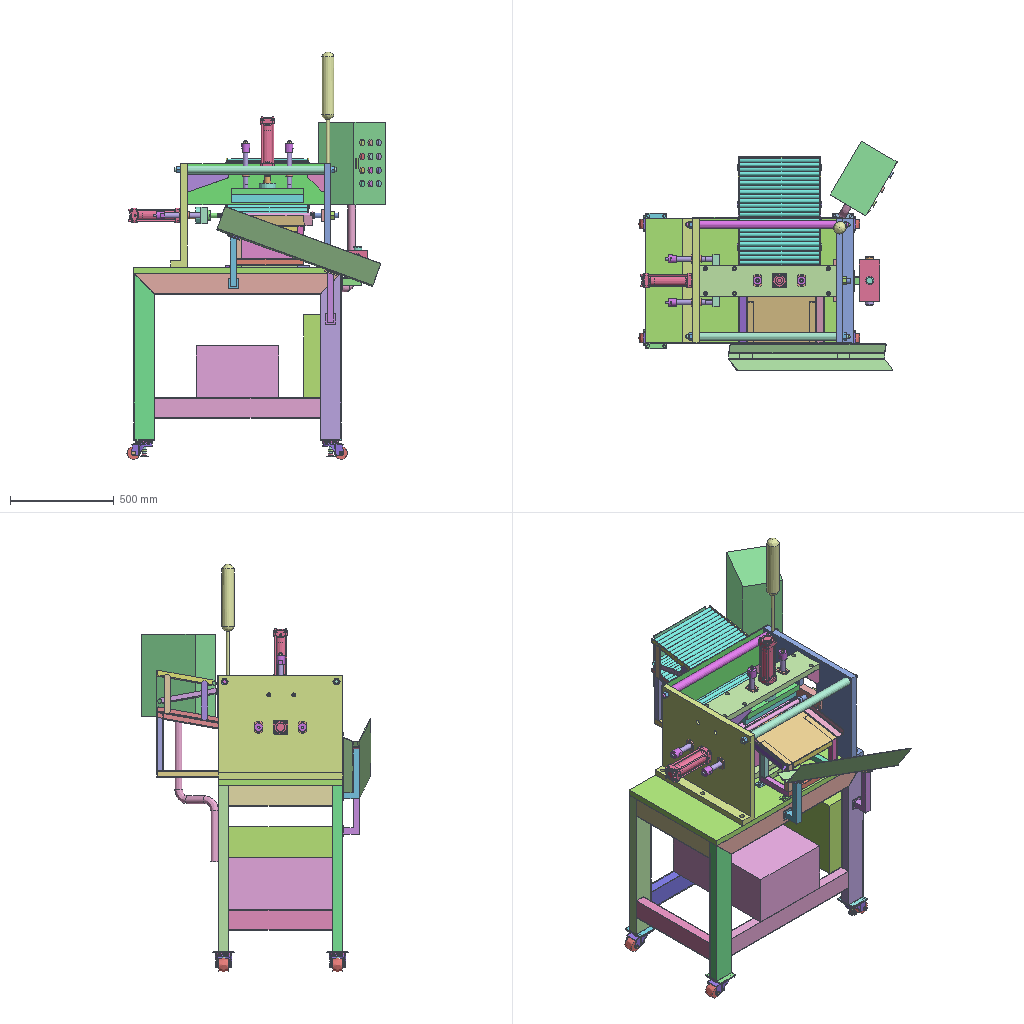Assembly | NX | 59 different items | 147 placed | box 1246 x 1107 x 1967 mm
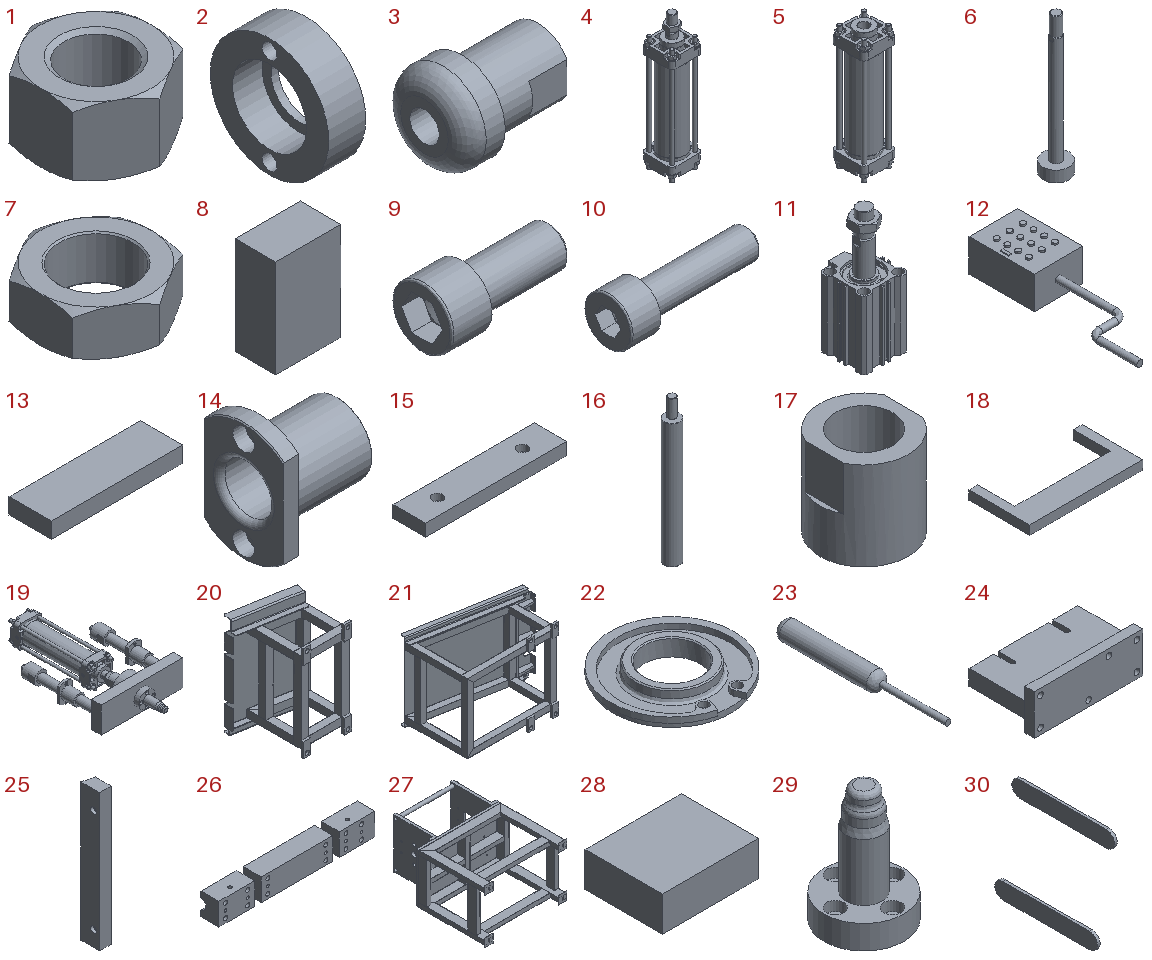Parts list (item | quantity | parent item | size | volume | features):
1 | x1 | in 53 | 36 x 41.569 x 22.3 mm | 17091 mm3 | features Hexagon Nut ISO - 4034 - M24 - N_Hexagon Nut ISO - 4034 - M24 - N 2
2 | x2 | in 19, 52 | 25 x 80 x 80 mm | 76796 mm3 | features Hydraulic support1 2
3 | x2 | in 19, 52 | 60 x 45 x 45 mm | 53203 mm3 | features Hydraulic support2 2
4 | x2 | in 19, 52 | 70 x 70 x 309 mm | 532464 mm3 | features Hydraulic2.1_50 2, Hydraulic2.2_50 2, Hydraulic2.3_M18X1.5 2
5 | x2 | in 4 | 70 x 70 x 262 mm | 413187 mm3 | features Hydraulic2.1_50 2
6 | x2 | in 4 | 50 x 50 x 263.5 mm | 115173 mm3 | features Hydraulic2.2_50 2
7 | x2 | in 4 | 27.02 x 31.2 x 11 mm | 4104 mm3 | features Hydraulic2.3_M18X1.5 2
8 | x1 | in 51 | 400 x 250 x 600 mm | 60000000 mm3 | features Hydrolic power unit 2
9 | x2 | in 52 | 51 x 24 x 24 mm | 12640 mm3 | features ISO 4762 M16 x 35 --- 35N_ISO 4762 M16 x 35 --- 35N 2
10 | x12 | in 54 | 38 x 13 x 13 mm | 2417 mm3 | features ISO 4762 M8 x 30 --- 30N_ISO 4762 M8 x 30 --- 30N 2
11 | x1 | in 54 | 45 x 49.5 x 124.5 mm | 95190 mm3 | features CDQ2B32-35DM_CQ2 SnapRing_32 2, CDQ2B32-35DM_CQ22031Rods_32M 2, CDQ2B32-35DM_CQ2Tube_32B 2, CDQ2B32-35DM_RodEndNuts_M14X1.5 2
12 | x1 | in 51 | 369 x 1100 x 210 mm | 25060594 mm3 | features Panel 16
13 | x1 | in 19 | 250 x 80 x 30 mm | 600000 mm3 | features Part2 2
14 | x4 | in 19, 52 | 48 x 40 x 60 mm | 31044 mm3 | features bushing 2
15 | x1 | in 52 | 350 x 80 x 30 mm | 816275 mm3 | features clamp plate 2
16 | x4 | in 19, 52 | 25 x 25 x 230 mm | 95439 mm3 | features clamp shaft 2
17 | x4 | in 19, 52 | 40 x 40 x 40 mm | 32581 mm3 | features clamp stopper 2
18 | x1 | in 54 | 190 x 102.2 x 15 mm | 141990 mm3 | features ejector support 2
19 | x1 | in 53 | 250 x 451 x 80 mm | 1627599 mm3 | features Hydraulic support1 2, Hydraulic support2 2, Hydraulic2.1_50 2, Hydraulic2.2_50 2, Hydraulic2.3_M18X1.5 2, Part2 2, bushing 2, clamp shaft 2, clamp stopper 2, mandrel expand 2
20 | x1 | in 51 | 278.549 x 270.487 x 416 mm | 850854 mm3 | features guide rail pipe2_Default_As Machined_ 20
21 | x1 | in 56 | 542.513 x 348.38 x 410 mm | 1580217 mm3 | features guide rail pipe_Default_As Machined_ 24
22 | x1 | in 11 | 35.7 x 35.209 x 4.9 mm | 1920 mm3 | features CDQ2B32-35DM_CQ2 SnapRing_32 2
23 | x1 | in 51 | 59.62 x 537.38 x 59.62 mm | 918566 mm3 | features information lamp 2
24 | x1 | in 54 | 350 x 210 x 130 mm | 4381610 mm3 | features lower clamp stand 3
25 | x1 | in 54 | 29.5 x 47.905 x 350 mm | 448357 mm3 | features lower clamp support 2, MOVE_FACE 1
26 | x1 | in 54 | 350 x 40 x 50 mm | 508342 mm3 | features lower clamp 4
27 | x1 | in 51 | 1000 x 1335 x 650 mm | 44393432 mm3 | features main frame_Default_As Machined_ 25
28 | x1 | in 51 | 500 x 400 x 180 mm | 36000000 mm3 | features main panel 2
29 | x1 | in 19 | 50 x 50 x 78 mm | 47044 mm3 | features mandrel expand 2
30 | x2 | in 56 | 5 x 223.069 x 210 mm | 55468 mm3 | features material feeder support 3
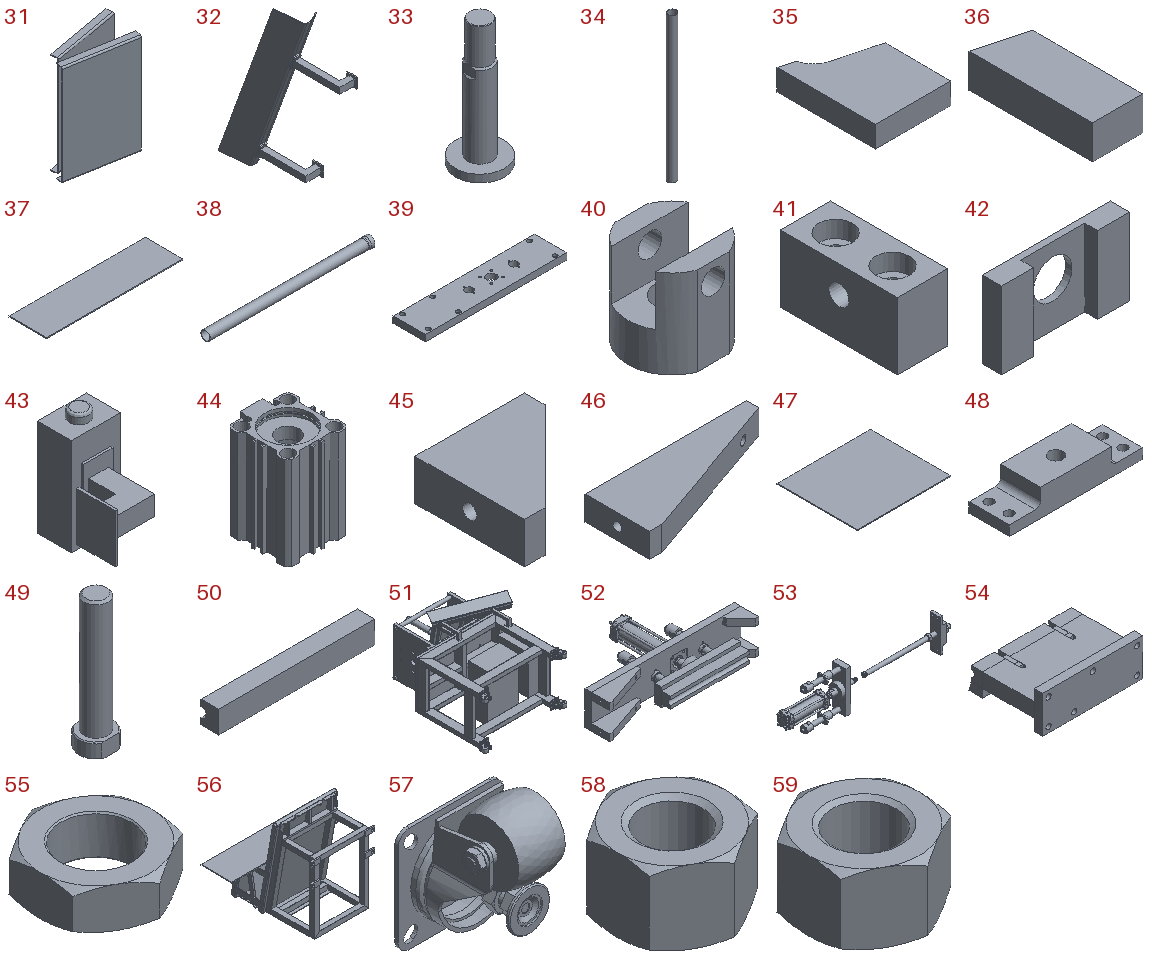31 | x1 | in 56 | 291.042 x 161.028 x 396 mm | 713843 mm3 | features material feeder 3
32 | x1 | in 51 | 134.94 x 565.526 x 791.184 mm | 1060388 mm3 | features output director 8
33 | x1 | in 11 | 32 x 32 x 82.5 mm | 18409 mm3 | features CDQ2B32-35DM_CQ22031Rods_32M 2
34 | x50 | in 56 | 22.2 x 22.2 x 385 mm | 30480 mm3 | features pipe belum expand 2
35 | x2 | in 54 | 49.5 x 64.866 x 14 mm | 36068 mm3 | features MOVE_FACE 3, pipe ejector 2
36 | x2 | in 54 | 22.2 x 55 x 15 mm | 17325 mm3 | features pipe injector 2
37 | x1 | in 56 | 723 x 200 x 5 mm | 723000 mm3 | features pipe partition 2
38 | x1 | in 53 | 385 x 24.9 x 24.9 mm | 30600 mm3 | features pipe setelah expand 2
39 | x1 | in 52 | - | 2805404 mm3 | features plate 2
40 | x1 | in 54 | 30 x 28 x 30 mm | 11330 mm3 | features pneumatic support1 2
41 | x1 | in 54 | 15 x 35 x 20 mm | 8578 mm3 | features pneumatic support2 2
42 | x1 | in 54 | 100 x 15 x 60 mm | 56466 mm3 | features pneumatic support 2
43 | x1 | in 51 | 130 x 210 x 236 mm | 1605041 mm3 | features push bottom 6
44 | x1 | in 11 | 45 x 49.5 x 68 mm | 72766 mm3 | features CDQ2B32-35DM_CQ2Tube_32B 2
45 | x2 | in 52 | - | 123670 mm3 | features stifener1 2
46 | x2 | in 52 | - | 292583 mm3 | features stifener2 2
47 | x1 | in 56 | 350 x 300 x 3 mm | 315000 mm3 | features stopper partition 2
48 | x1 | in 53 | 200 x 60 x 40 mm | 317330 mm3 | features stopper pipe support 2
49 | x1 | in 53 | 35 x 30 x 135 mm | 67591 mm3 | features stopper pipe 2
50 | x1 | in 52 | 350 x 40 x 50 mm | 632262 mm3 | features upper clamp 2
51 | x1 | - | 1246 x 1967 x 1107 mm | 170914110 mm3 | features main frame_Default_As Machined_ 25, guide rail pipe2_Default_As Machined_ 20, Panel 16, CMAS65-F 12, output director 8, push bottom 6, Hexagon Nut ISO - 4034 - M20 - N_Hexagon Nut ISO - 4034 - M20 - N 2, Hydrolic power unit 2, information lamp 2, main panel 2
52 | x1 | - | - | 6097092 mm3 | features Hexagon Nut ISO - 4034 - M12 - N_Hexagon Nut ISO - 4034 - M12 - N 2, Hydraulic support1 2, Hydraulic support2 2, Hydraulic2.1_50 2, Hydraulic2.2_50 2, Hydraulic2.3_M18X1.5 2, ISO 4762 M16 x 35 --- 35N_ISO 4762 M16 x 35 --- 35N 2, bushing 2, clamp plate 2, clamp shaft 2, clamp stopper 2, plate 2, stifener1 2, stifener2 2, upper clamp 2
53 | x1 | - | 1014 x 80 x 250 mm | 2060226 mm3 | features Hexagon Nut ISO - 4034 - M24 - N_Hexagon Nut ISO - 4034 - M24 - N 2, Hydraulic support1 2, Hydraulic support2 2, Hydraulic2.1_50 2, Hydraulic2.2_50 2, Hydraulic2.3_M18X1.5 2, Part2 2, bushing 2, clamp shaft 2, clamp stopper 2, mandrel expand 2, pipe setelah expand 2, stopper pipe 2, stopper pipe support 2
54 | x1 | - | 350 x 257.905 x 151.7 mm | 5787641 mm3 | features MOVE_FACE 4, lower clamp 4, lower clamp stand 3, CDQ2B32-35DM_CQ2 SnapRing_32 2, CDQ2B32-35DM_CQ22031Rods_32M 2, CDQ2B32-35DM_CQ2Tube_32B 2, CDQ2B32-35DM_RodEndNuts_M14X1.5 2, ISO 4762 M8 x 30 --- 30N_ISO 4762 M8 x 30 --- 30N 2, ejector support 2, lower clamp support 2, pipe ejector 2, pipe injector 2, pneumatic support 2, pneumatic support1 2, pneumatic support2 2
55 | x1 | in 11 | 21.997 x 25.4 x 8 mm | 2094 mm3 | features CDQ2B32-35DM_RodEndNuts_M14X1.5 2
56 | x1 | - | 723 x 525.58 x 545.165 mm | 4966986 mm3 | features guide rail pipe_Default_As Machined_ 24, material feeder 3, material feeder support 3, pipe belum expand 2, pipe partition 2, stopper partition 2
57 | x4 | in 51 | 102 x 113.8 x 134.5 mm | 246246 mm3 | features CMAS65-F 12
58 | x2 | in 52 | 18 x 20.785 x 12.2 mm | 2393 mm3 | features Hexagon Nut ISO - 4034 - M12 - N_Hexagon Nut ISO - 4034 - M12 - N 2
59 | x4 | in 51 | 30 x 34.641 x 19 mm | 10115 mm3 | features Hexagon Nut ISO - 4034 - M20 - N_Hexagon Nut ISO - 4034 - M20 - N 2